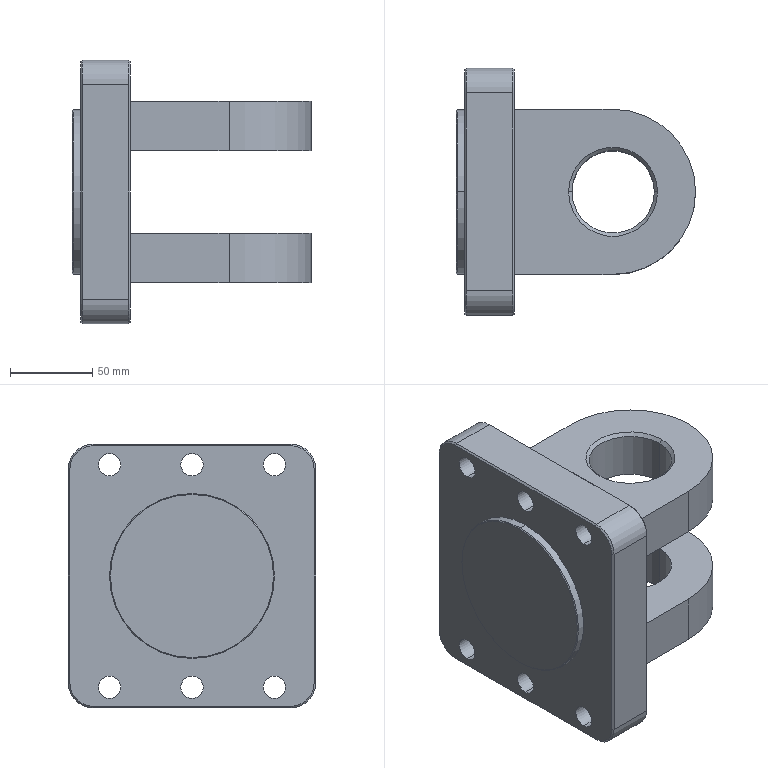Part | SolidWorks | features Chamfer 4, ICE 3, Fillet 2, Extrusion 1, HoleWzd 1, MirrorPattern 1 | 1 solid | 81 faces | box 145 x 150 x 160 mm | volume 1190904 mm3 | cylinder 38 | plane 29 | cone 14 | commonest cylinder face diameters 13.5 x12 20 x12 100 x6 30 x4 50 x4